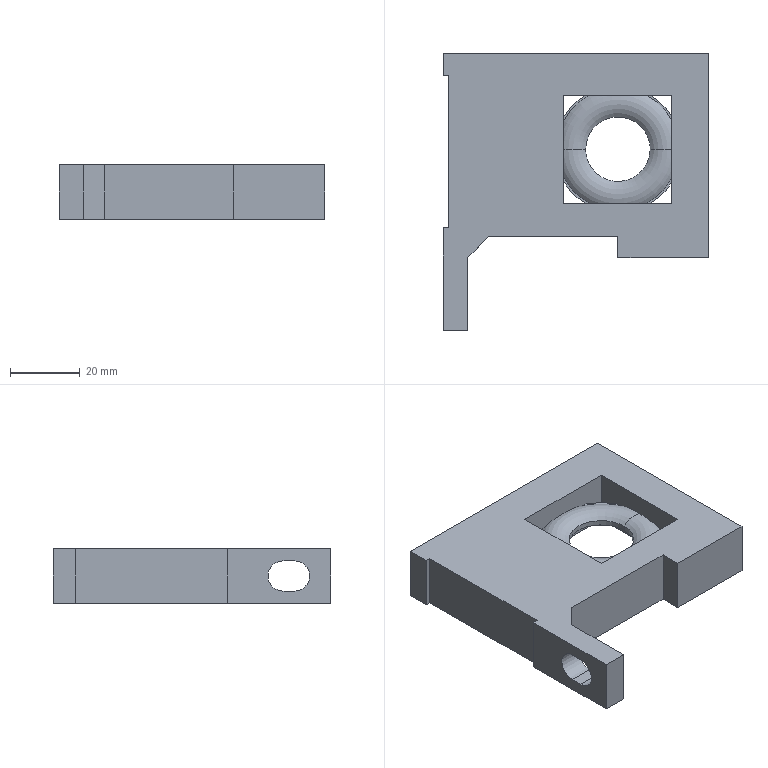Part | SolidWorks | features BaseBody 1 | 1 solid | 57 faces | box 76 x 79.5 x 15.5 mm | volume 53255 mm3 | plane 33 | cylinder 16 | torus 8 | commonest cylinder face diameters 8.5 x4 9 x4 36.2 x4 8.6 x2 18.5 x2